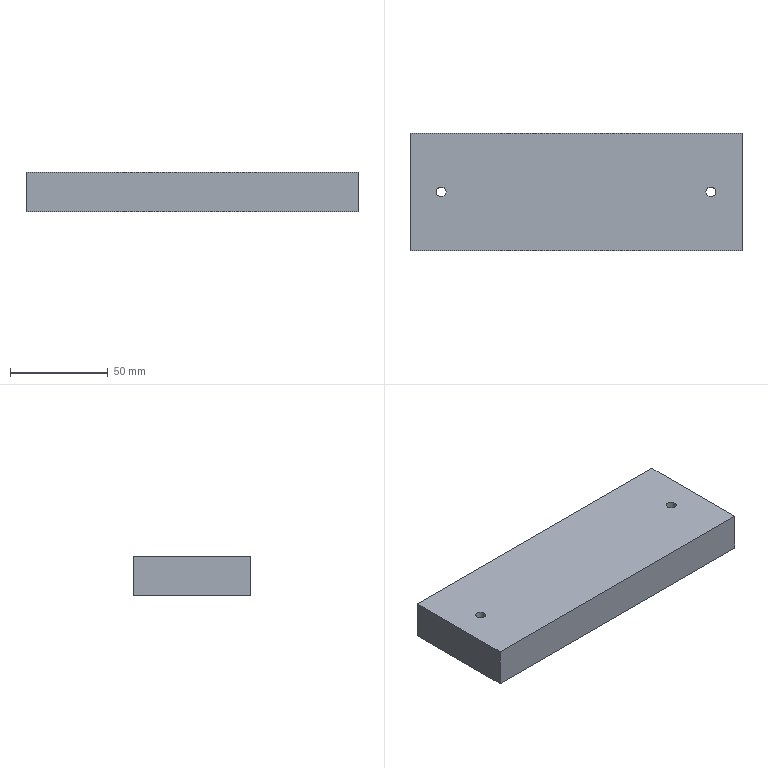Part | NX | 1 solid | 24 faces | box 170 x 60 x 20 mm | volume 202900 mm3 | plane 10 | torus 8 | cone 4 | cylinder 2 | commonest cylinder face diameters 5 x2
STEP:
#1=CARTESIAN_POINT('',(-85.,30.,1.5));
#2=VERTEX_POINT('',#1);
#3=CARTESIAN_POINT('',(-85.,-30.,1.5));
#4=VERTEX_POINT('',#3);
#5=CARTESIAN_POINT('',(-85.,28.565,1.5));
#6=DIRECTION('',(0.,-1.,0.));
#7=VECTOR('',#6,1000.);
#8=LINE('',#5,#7);
#9=EDGE_CURVE('',#2,#4,#8,.T.);
#10=ORIENTED_EDGE('',*,*,#9,.T.);
#11=CARTESIAN_POINT('',(-85.,-30.,21.5));
#12=VERTEX_POINT('',#11);
#13=CARTESIAN_POINT('',(-85.,-30.,1.5));
#14=DIRECTION('',(0.,0.,1.));
#15=VECTOR('',#14,1000.);
#16=LINE('',#13,#15);
#17=EDGE_CURVE('',#4,#12,#16,.T.);
#18=ORIENTED_EDGE('',*,*,#17,.T.);
#19=CARTESIAN_POINT('',(-85.,30.,21.5));
#20=VERTEX_POINT('',#19);
#21=CARTESIAN_POINT('',(-85.,0.,21.5));
#22=DIRECTION('',(0.,1.,0.));
#23=VECTOR('',#22,1000.);
#24=LINE('',#21,#23);
#25=EDGE_CURVE('',#12,#20,#24,.T.);
#26=ORIENTED_EDGE('',*,*,#25,.T.);
#27=CARTESIAN_POINT('',(-85.,30.,1.5));
#28=DIRECTION('',(0.,0.,1.));
#29=VECTOR('',#28,1000.);
#30=LINE('',#27,#29);
#31=EDGE_CURVE('',#2,#20,#30,.T.);
#32=ORIENTED_EDGE('',*,*,#31,.F.);
#33=EDGE_LOOP('',(#10,#18,#26,#32));
#34=FACE_BOUND('',#33,.T.);
#35=CARTESIAN_POINT('',(-85.,0.,1.5));
#36=DIRECTION('',(-1.,0.,0.));
#37=DIRECTION('',(0.,0.,1.));
#38=AXIS2_PLACEMENT_3D('',#35,#36,#37);
#39=PLANE('',#38);
#40=ADVANCED_FACE('',(#34),#39,.T.);
#41=CARTESIAN_POINT('',(85.,-30.,1.5));
#42=VERTEX_POINT('',#41);
#43=CARTESIAN_POINT('',(85.,30.,1.5));
#44=VERTEX_POINT('',#43);
#45=CARTESIAN_POINT('',(85.,28.565,1.5));
#46=DIRECTION('',(0.,1.,0.));
#47=VECTOR('',#46,1000.);
#48=LINE('',#45,#47);
#49=EDGE_CURVE('',#42,#44,#48,.T.);
#50=ORIENTED_EDGE('',*,*,#49,.T.);
#51=CARTESIAN_POINT('',(85.,30.,21.5));
#52=VERTEX_POINT('',#51);
#53=CARTESIAN_POINT('',(85.,30.,1.5));
#54=DIRECTION('',(0.,0.,1.));
#55=VECTOR('',#54,1000.);
#56=LINE('',#53,#55);
#57=EDGE_CURVE('',#44,#52,#56,.T.);
#58=ORIENTED_EDGE('',*,*,#57,.T.);
#59=CARTESIAN_POINT('',(85.,-30.,21.5));
#60=VERTEX_POINT('',#59);
#61=CARTESIAN_POINT('',(85.,0.,21.5));
#62=DIRECTION('',(0.,-1.,0.));
#63=VECTOR('',#62,1000.);
#64=LINE('',#61,#63);
#65=EDGE_CURVE('',#52,#60,#64,.T.);
#66=ORIENTED_EDGE('',*,*,#65,.T.);
#67=CARTESIAN_POINT('',(85.,-30.,1.5));
#68=DIRECTION('',(0.,0.,1.));
#69=VECTOR('',#68,1000.);
#70=LINE('',#67,#69);
#71=EDGE_CURVE('',#42,#60,#70,.T.);
#72=ORIENTED_EDGE('',*,*,#71,.F.);
#73=EDGE_LOOP('',(#50,#58,#66,#72));
#74=FACE_BOUND('',#73,.T.);
#75=CARTESIAN_POINT('',(85.,0.,1.5));
#76=DIRECTION('',(1.,0.,0.));
#77=DIRECTION('',(0.,0.,-1.));
#78=AXIS2_PLACEMENT_3D('',#75,#76,#77);
#79=PLANE('',#78);
#80=ADVANCED_FACE('',(#74),#79,.T.);
#81=CARTESIAN_POINT('',(71.5,0.,21.5));
#82=VERTEX_POINT('',#81);
#83=CARTESIAN_POINT('',(69.,0.,21.5));
#84=DIRECTION('',(0.,0.,1.));
#85=DIRECTION('',(1.,0.,0.));
#86=AXIS2_PLACEMENT_3D('',#83,#84,#85);
#87=CIRCLE('',#86,2.5);
#88=EDGE_CURVE('',#82,#82,#87,.F.);
#89=ORIENTED_EDGE('',*,*,#88,.T.);
#90=EDGE_LOOP('',(#89));
#91=FACE_BOUND('',#90,.T.);
#92=CARTESIAN_POINT('',(-66.5,0.,21.5));
#93=VERTEX_POINT('',#92);
#94=CARTESIAN_POINT('',(-69.,0.,21.5));
#95=DIRECTION('',(0.,0.,1.));
#96=DIRECTION('',(1.,0.,0.));
#97=AXIS2_PLACEMENT_3D('',#94,#95,#96);
#98=CIRCLE('',#97,2.5);
#99=EDGE_CURVE('',#93,#93,#98,.F.);
#100=ORIENTED_EDGE('',*,*,#99,.T.);
#101=EDGE_LOOP('',(#100));
#102=FACE_BOUND('',#101,.T.);
#103=CARTESIAN_POINT('',(0.,-30.,21.5));
#104=DIRECTION('',(-1.,0.,0.));
#105=VECTOR('',#104,1000.);
#106=LINE('',#103,#105);
#107=EDGE_CURVE('',#60,#12,#106,.T.);
#108=ORIENTED_EDGE('',*,*,#107,.F.);
#109=ORIENTED_EDGE('',*,*,#65,.F.);
#110=CARTESIAN_POINT('',(0.,30.,21.5));
#111=DIRECTION('',(1.,0.,0.));
#112=VECTOR('',#111,1000.);
#113=LINE('',#110,#112);
#114=EDGE_CURVE('',#20,#52,#113,.T.);
#115=ORIENTED_EDGE('',*,*,#114,.F.);
#116=ORIENTED_EDGE('',*,*,#25,.F.);
#117=EDGE_LOOP('',(#108,#109,#115,#116));
#118=FACE_BOUND('',#117,.T.);
#119=CARTESIAN_POINT('',(0.,0.,21.5));
#120=DIRECTION('',(0.,0.,1.));
#121=DIRECTION('',(1.,0.,0.));
#122=AXIS2_PLACEMENT_3D('',#119,#120,#121);
#123=PLANE('',#122);
#124=ADVANCED_FACE('',(#91,#102,#118),#123,.T.);
#125=CARTESIAN_POINT('',(-38.195,15.,1.5));
#126=VERTEX_POINT('',#125);
#127=CARTESIAN_POINT('',(-41.999,15.,1.5));
#128=DIRECTION('',(0.,0.,1.));
#129=DIRECTION('',(1.,0.,0.));
#130=AXIS2_PLACEMENT_3D('',#127,#128,#129);
#131=CIRCLE('',#130,3.804);
#132=EDGE_CURVE('',#126,#126,#131,.T.);
#133=ORIENTED_EDGE('',*,*,#132,.T.);
#134=EDGE_LOOP('',(#133));
#135=FACE_BOUND('',#134,.T.);
#136=CARTESIAN_POINT('',(45.805,15.,1.5));
#137=VERTEX_POINT('',#136);
#138=CARTESIAN_POINT('',(42.001,15.,1.5));
#139=DIRECTION('',(0.,0.,1.));
#140=DIRECTION('',(1.,0.,0.));
#141=AXIS2_PLACEMENT_3D('',#138,#139,#140);
#142=CIRCLE('',#141,3.804);
#143=EDGE_CURVE('',#137,#137,#142,.T.);
#144=ORIENTED_EDGE('',*,*,#143,.T.);
#145=EDGE_LOOP('',(#144));
#146=FACE_BOUND('',#145,.T.);
#147=CARTESIAN_POINT('',(28.805,-22.,1.5));
#148=VERTEX_POINT('',#147);
#149=CARTESIAN_POINT('',(25.001,-22.,1.5));
#150=DIRECTION('',(0.,0.,1.));
#151=DIRECTION('',(1.,0.,0.));
#152=AXIS2_PLACEMENT_3D('',#149,#150,#151);
#153=CIRCLE('',#152,3.804);
#154=EDGE_CURVE('',#148,#148,#153,.T.);
#155=ORIENTED_EDGE('',*,*,#154,.T.);
#156=EDGE_LOOP('',(#155));
#157=FACE_BOUND('',#156,.T.);
#158=CARTESIAN_POINT('',(-21.195,-22.,1.5));
#159=VERTEX_POINT('',#158);
#160=CARTESIAN_POINT('',(-24.999,-22.,1.5));
#161=DIRECTION('',(0.,0.,1.));
#162=DIRECTION('',(1.,0.,0.));
#163=AXIS2_PLACEMENT_3D('',#160,#161,#162);
#164=CIRCLE('',#163,3.804);
#165=EDGE_CURVE('',#159,#159,#164,.T.);
#166=ORIENTED_EDGE('',*,*,#165,.T.);
#167=EDGE_LOOP('',(#166));
#168=FACE_BOUND('',#167,.T.);
#169=CARTESIAN_POINT('',(71.5,0.,1.5));
#170=VERTEX_POINT('',#169);
#171=CARTESIAN_POINT('',(69.,0.,1.5));
#172=DIRECTION('',(0.,0.,1.));
#173=DIRECTION('',(1.,0.,0.));
#174=AXIS2_PLACEMENT_3D('',#171,#172,#173);
#175=CIRCLE('',#174,2.5);
#176=EDGE_CURVE('',#170,#170,#175,.T.);
#177=ORIENTED_EDGE('',*,*,#176,.T.);
#178=EDGE_LOOP('',(#177));
#179=FACE_BOUND('',#178,.T.);
#180=CARTESIAN_POINT('',(-66.5,0.,1.5));
#181=VERTEX_POINT('',#180);
#182=CARTESIAN_POINT('',(-69.,0.,1.5));
#183=DIRECTION('',(0.,0.,1.));
#184=DIRECTION('',(1.,0.,0.));
#185=AXIS2_PLACEMENT_3D('',#182,#183,#184);
#186=CIRCLE('',#185,2.5);
#187=EDGE_CURVE('',#181,#181,#186,.T.);
#188=ORIENTED_EDGE('',*,*,#187,.T.);
#189=EDGE_LOOP('',(#188));
#190=FACE_BOUND('',#189,.T.);
#191=CARTESIAN_POINT('',(0.,-30.,1.5));
#192=DIRECTION('',(1.,0.,0.));
#193=VECTOR('',#192,1000.);
#194=LINE('',#191,#193);
#195=EDGE_CURVE('',#4,#42,#194,.T.);
#196=ORIENTED_EDGE('',*,*,#195,.F.);
#197=ORIENTED_EDGE('',*,*,#9,.F.);
#198=CARTESIAN_POINT('',(0.,30.,1.5));
#199=DIRECTION('',(-1.,0.,0.));
#200=VECTOR('',#199,1000.);
#201=LINE('',#198,#200);
#202=EDGE_CURVE('',#44,#2,#201,.T.);
#203=ORIENTED_EDGE('',*,*,#202,.F.);
#204=ORIENTED_EDGE('',*,*,#49,.F.);
#205=EDGE_LOOP('',(#196,#197,#203,#204));
#206=FACE_BOUND('',#205,.T.);
#207=CARTESIAN_POINT('',(44.401,28.565,1.5));
#208=DIRECTION('',(0.,0.,1.));
#209=DIRECTION('',(1.,0.,0.));
#210=AXIS2_PLACEMENT_3D('',#207,#208,#209);
#211=PLANE('',#210);
#212=ADVANCED_FACE('',(#135,#146,#157,#168,#179,#190,#206),#211,.F.);
#213=CARTESIAN_POINT('',(-23.637,-22.,6.5));
#214=VERTEX_POINT('',#213);
#215=CARTESIAN_POINT('',(-24.999,-22.,6.5));
#216=DIRECTION('',(0.,0.,1.));
#217=DIRECTION('',(1.,0.,0.));
#218=AXIS2_PLACEMENT_3D('',#215,#216,#217);
#219=CIRCLE('',#218,1.363);
#220=EDGE_CURVE('',#214,#214,#219,.F.);
#221=ORIENTED_EDGE('',*,*,#220,.T.);
#222=EDGE_LOOP('',(#221));
#223=FACE_BOUND('',#222,.T.);
#224=CARTESIAN_POINT('',(-24.999,-22.,6.5));
#225=DIRECTION('',(0.,0.,1.));
#226=DIRECTION('',(0.,1.,0.));
#227=AXIS2_PLACEMENT_3D('',#224,#225,#226);
#228=PLANE('',#227);
#229=ADVANCED_FACE('',(#223),#228,.F.);
#230=CARTESIAN_POINT('',(-26.857,-22.,6.07));
#231=VERTEX_POINT('',#230);
#232=CARTESIAN_POINT('',(-24.999,-22.,6.07));
#233=DIRECTION('',(0.,0.,-1.));
#234=DIRECTION('',(-1.,0.,0.));
#235=AXIS2_PLACEMENT_3D('',#232,#233,#234);
#236=CIRCLE('',#235,1.858);
#237=EDGE_CURVE('',#231,#231,#236,.F.);
#238=ORIENTED_EDGE('',*,*,#237,.T.);
#239=EDGE_LOOP('',(#238));
#240=FACE_BOUND('',#239,.T.);
#241=CARTESIAN_POINT('',(-22.681,-22.,2.791));
#242=VERTEX_POINT('',#241);
#243=CARTESIAN_POINT('',(-24.999,-22.,2.791));
#244=DIRECTION('',(0.,0.,1.));
#245=DIRECTION('',(1.,0.,0.));
#246=AXIS2_PLACEMENT_3D('',#243,#244,#245);
#247=CIRCLE('',#246,2.319);
#248=EDGE_CURVE('',#242,#242,#247,.F.);
#249=ORIENTED_EDGE('',*,*,#248,.T.);
#250=EDGE_LOOP('',(#249));
#251=FACE_BOUND('',#250,.T.);
#252=CARTESIAN_POINT('',(-24.999,-22.,1.5));
#253=DIRECTION('',(0.,0.,-1.));
#254=DIRECTION('',(0.,1.,0.));
#255=AXIS2_PLACEMENT_3D('',#252,#253,#254);
#256=CONICAL_SURFACE('',#255,2.5,0.1396);
#257=ADVANCED_FACE('',(#240,#251),#256,.F.);
#258=CARTESIAN_POINT('',(26.363,-22.,6.5));
#259=VERTEX_POINT('',#258);
#260=CARTESIAN_POINT('',(25.001,-22.,6.5));
#261=DIRECTION('',(0.,0.,1.));
#262=DIRECTION('',(1.,0.,0.));
#263=AXIS2_PLACEMENT_3D('',#260,#261,#262);
#264=CIRCLE('',#263,1.363);
#265=EDGE_CURVE('',#259,#259,#264,.F.);
#266=ORIENTED_EDGE('',*,*,#265,.T.);
#267=EDGE_LOOP('',(#266));
#268=FACE_BOUND('',#267,.T.);
#269=CARTESIAN_POINT('',(25.001,-22.,6.5));
#270=DIRECTION('',(0.,0.,1.));
#271=DIRECTION('',(0.,1.,0.));
#272=AXIS2_PLACEMENT_3D('',#269,#270,#271);
#273=PLANE('',#272);
#274=ADVANCED_FACE('',(#268),#273,.F.);
#275=CARTESIAN_POINT('',(23.143,-22.,6.07));
#276=VERTEX_POINT('',#275);
#277=CARTESIAN_POINT('',(25.001,-22.,6.07));
#278=DIRECTION('',(0.,0.,-1.));
#279=DIRECTION('',(-1.,0.,0.));
#280=AXIS2_PLACEMENT_3D('',#277,#278,#279);
#281=CIRCLE('',#280,1.858);
#282=EDGE_CURVE('',#276,#276,#281,.F.);
#283=ORIENTED_EDGE('',*,*,#282,.T.);
#284=EDGE_LOOP('',(#283));
#285=FACE_BOUND('',#284,.T.);
#286=CARTESIAN_POINT('',(27.319,-22.,2.791));
#287=VERTEX_POINT('',#286);
#288=CARTESIAN_POINT('',(25.001,-22.,2.791));
#289=DIRECTION('',(0.,0.,1.));
#290=DIRECTION('',(1.,0.,0.));
#291=AXIS2_PLACEMENT_3D('',#288,#289,#290);
#292=CIRCLE('',#291,2.319);
#293=EDGE_CURVE('',#287,#287,#292,.F.);
#294=ORIENTED_EDGE('',*,*,#293,.T.);
#295=EDGE_LOOP('',(#294));
#296=FACE_BOUND('',#295,.T.);
#297=CARTESIAN_POINT('',(25.001,-22.,1.5));
#298=DIRECTION('',(0.,0.,-1.));
#299=DIRECTION('',(0.,1.,0.));
#300=AXIS2_PLACEMENT_3D('',#297,#298,#299);
#301=CONICAL_SURFACE('',#300,2.5,0.1396);
#302=ADVANCED_FACE('',(#285,#296),#301,.F.);
#303=CARTESIAN_POINT('',(40.638,15.,6.5));
#304=VERTEX_POINT('',#303);
#305=CARTESIAN_POINT('',(42.001,15.,6.5));
#306=DIRECTION('',(0.,0.,-1.));
#307=DIRECTION('',(-1.,0.,0.));
#308=AXIS2_PLACEMENT_3D('',#305,#306,#307);
#309=CIRCLE('',#308,1.363);
#310=EDGE_CURVE('',#304,#304,#309,.T.);
#311=ORIENTED_EDGE('',*,*,#310,.T.);
#312=EDGE_LOOP('',(#311));
#313=FACE_BOUND('',#312,.T.);
#314=CARTESIAN_POINT('',(42.001,15.,6.5));
#315=DIRECTION('',(0.,0.,-1.));
#316=DIRECTION('',(0.,-1.,0.));
#317=AXIS2_PLACEMENT_3D('',#314,#315,#316);
#318=PLANE('',#317);
#319=ADVANCED_FACE('',(#313),#318,.T.);
#320=CARTESIAN_POINT('',(43.859,15.,6.07));
#321=VERTEX_POINT('',#320);
#322=CARTESIAN_POINT('',(42.001,15.,6.07));
#323=DIRECTION('',(0.,0.,1.));
#324=DIRECTION('',(1.,0.,0.));
#325=AXIS2_PLACEMENT_3D('',#322,#323,#324);
#326=CIRCLE('',#325,1.858);
#327=EDGE_CURVE('',#321,#321,#326,.T.);
#328=ORIENTED_EDGE('',*,*,#327,.T.);
#329=EDGE_LOOP('',(#328));
#330=FACE_BOUND('',#329,.T.);
#331=CARTESIAN_POINT('',(44.319,15.,2.791));
#332=VERTEX_POINT('',#331);
#333=CARTESIAN_POINT('',(42.001,15.,2.791));
#334=DIRECTION('',(0.,0.,1.));
#335=DIRECTION('',(1.,0.,0.));
#336=AXIS2_PLACEMENT_3D('',#333,#334,#335);
#337=CIRCLE('',#336,2.319);
#338=EDGE_CURVE('',#332,#332,#337,.F.);
#339=ORIENTED_EDGE('',*,*,#338,.T.);
#340=EDGE_LOOP('',(#339));
#341=FACE_BOUND('',#340,.T.);
#342=CARTESIAN_POINT('',(42.001,15.,1.5));
#343=DIRECTION('',(0.,0.,-1.));
#344=DIRECTION('',(0.,1.,0.));
#345=AXIS2_PLACEMENT_3D('',#342,#343,#344);
#346=CONICAL_SURFACE('',#345,2.5,0.1396);
#347=ADVANCED_FACE('',(#330,#341),#346,.F.);
#348=CARTESIAN_POINT('',(-40.637,15.,6.5));
#349=VERTEX_POINT('',#348);
#350=CARTESIAN_POINT('',(-41.999,15.,6.5));
#351=DIRECTION('',(0.,0.,1.));
#352=DIRECTION('',(1.,0.,0.));
#353=AXIS2_PLACEMENT_3D('',#350,#351,#352);
#354=CIRCLE('',#353,1.363);
#355=EDGE_CURVE('',#349,#349,#354,.F.);
#356=ORIENTED_EDGE('',*,*,#355,.T.);
#357=EDGE_LOOP('',(#356));
#358=FACE_BOUND('',#357,.T.);
#359=CARTESIAN_POINT('',(-41.999,15.,6.5));
#360=DIRECTION('',(0.,0.,1.));
#361=DIRECTION('',(0.,1.,0.));
#362=AXIS2_PLACEMENT_3D('',#359,#360,#361);
#363=PLANE('',#362);
#364=ADVANCED_FACE('',(#358),#363,.F.);
#365=CARTESIAN_POINT('',(-43.857,15.,6.07));
#366=VERTEX_POINT('',#365);
#367=CARTESIAN_POINT('',(-41.999,15.,6.07));
#368=DIRECTION('',(0.,0.,-1.));
#369=DIRECTION('',(-1.,0.,0.));
#370=AXIS2_PLACEMENT_3D('',#367,#368,#369);
#371=CIRCLE('',#370,1.858);
#372=EDGE_CURVE('',#366,#366,#371,.F.);
#373=ORIENTED_EDGE('',*,*,#372,.T.);
#374=EDGE_LOOP('',(#373));
#375=FACE_BOUND('',#374,.T.);
#376=CARTESIAN_POINT('',(-39.681,15.,2.791));
#377=VERTEX_POINT('',#376);
#378=CARTESIAN_POINT('',(-41.999,15.,2.791));
#379=DIRECTION('',(0.,0.,1.));
#380=DIRECTION('',(1.,0.,0.));
#381=AXIS2_PLACEMENT_3D('',#378,#379,#380);
#382=CIRCLE('',#381,2.319);
#383=EDGE_CURVE('',#377,#377,#382,.F.);
#384=ORIENTED_EDGE('',*,*,#383,.T.);
#385=EDGE_LOOP('',(#384));
#386=FACE_BOUND('',#385,.T.);
#387=CARTESIAN_POINT('',(-41.999,15.,1.5));
#388=DIRECTION('',(0.,0.,-1.));
#389=DIRECTION('',(0.,1.,0.));
#390=AXIS2_PLACEMENT_3D('',#387,#388,#389);
#391=CONICAL_SURFACE('',#390,2.5,0.1396);
#392=ADVANCED_FACE('',(#375,#386),#391,.F.);
#393=ORIENTED_EDGE('',*,*,#31,.T.);
#394=ORIENTED_EDGE('',*,*,#114,.T.);
#395=ORIENTED_EDGE('',*,*,#57,.F.);
#396=ORIENTED_EDGE('',*,*,#202,.T.);
#397=EDGE_LOOP('',(#393,#394,#395,#396));
#398=FACE_BOUND('',#397,.T.);
#399=CARTESIAN_POINT('',(0.,30.,1.5));
#400=DIRECTION('',(0.,1.,0.));
#401=DIRECTION('',(0.,0.,1.));
#402=AXIS2_PLACEMENT_3D('',#399,#400,#401);
#403=PLANE('',#402);
#404=ADVANCED_FACE('',(#398),#403,.T.);
#405=ORIENTED_EDGE('',*,*,#71,.T.);
#406=ORIENTED_EDGE('',*,*,#107,.T.);
#407=ORIENTED_EDGE('',*,*,#17,.F.);
#408=ORIENTED_EDGE('',*,*,#195,.T.);
#409=EDGE_LOOP('',(#405,#406,#407,#408));
#410=FACE_BOUND('',#409,.T.);
#411=CARTESIAN_POINT('',(0.,-30.,1.5));
#412=DIRECTION('',(0.,-1.,0.));
#413=DIRECTION('',(0.,0.,-1.));
#414=AXIS2_PLACEMENT_3D('',#411,#412,#413);
#415=PLANE('',#414);
#416=ADVANCED_FACE('',(#410),#415,.T.);
#417=ORIENTED_EDGE('',*,*,#99,.F.);
#418=EDGE_LOOP('',(#417));
#419=FACE_BOUND('',#418,.T.);
#420=ORIENTED_EDGE('',*,*,#187,.F.);
#421=EDGE_LOOP('',(#420));
#422=FACE_BOUND('',#421,.T.);
#423=CARTESIAN_POINT('',(-69.,0.,41.5));
#424=DIRECTION('',(0.,0.,-1.));
#425=DIRECTION('',(-1.,0.,0.));
#426=AXIS2_PLACEMENT_3D('',#423,#424,#425);
#427=CYLINDRICAL_SURFACE('',#426,2.5);
#428=ADVANCED_FACE('',(#419,#422),#427,.F.);
#429=ORIENTED_EDGE('',*,*,#88,.F.);
#430=EDGE_LOOP('',(#429));
#431=FACE_BOUND('',#430,.T.);
#432=ORIENTED_EDGE('',*,*,#176,.F.);
#433=EDGE_LOOP('',(#432));
#434=FACE_BOUND('',#433,.T.);
#435=CARTESIAN_POINT('',(69.,0.,41.5));
#436=DIRECTION('',(0.,0.,-1.));
#437=DIRECTION('',(-1.,0.,0.));
#438=AXIS2_PLACEMENT_3D('',#435,#436,#437);
#439=CYLINDRICAL_SURFACE('',#438,2.5);
#440=ADVANCED_FACE('',(#431,#434),#439,.F.);
#441=ORIENTED_EDGE('',*,*,#132,.F.);
#442=EDGE_LOOP('',(#441));
#443=FACE_BOUND('',#442,.T.);
#444=ORIENTED_EDGE('',*,*,#383,.F.);
#445=EDGE_LOOP('',(#444));
#446=FACE_BOUND('',#445,.T.);
#447=CARTESIAN_POINT('',(-41.999,15.,3.));
#448=DIRECTION('',(0.,0.,1.));
#449=DIRECTION('',(1.,0.,0.));
#450=AXIS2_PLACEMENT_3D('',#447,#448,#449);
#451=TOROIDAL_SURFACE('',#450,3.804,1.5);
#452=ADVANCED_FACE('',(#443,#446),#451,.T.);
#453=ORIENTED_EDGE('',*,*,#143,.F.);
#454=EDGE_LOOP('',(#453));
#455=FACE_BOUND('',#454,.T.);
#456=ORIENTED_EDGE('',*,*,#338,.F.);
#457=EDGE_LOOP('',(#456));
#458=FACE_BOUND('',#457,.T.);
#459=CARTESIAN_POINT('',(42.001,15.,3.));
#460=DIRECTION('',(0.,0.,1.));
#461=DIRECTION('',(1.,0.,0.));
#462=AXIS2_PLACEMENT_3D('',#459,#460,#461);
#463=TOROIDAL_SURFACE('',#462,3.804,1.5);
#464=ADVANCED_FACE('',(#455,#458),#463,.T.);
#465=ORIENTED_EDGE('',*,*,#154,.F.);
#466=EDGE_LOOP('',(#465));
#467=FACE_BOUND('',#466,.T.);
#468=ORIENTED_EDGE('',*,*,#293,.F.);
#469=EDGE_LOOP('',(#468));
#470=FACE_BOUND('',#469,.T.);
#471=CARTESIAN_POINT('',(25.001,-22.,3.));
#472=DIRECTION('',(0.,0.,1.));
#473=DIRECTION('',(1.,0.,0.));
#474=AXIS2_PLACEMENT_3D('',#471,#472,#473);
#475=TOROIDAL_SURFACE('',#474,3.804,1.5);
#476=ADVANCED_FACE('',(#467,#470),#475,.T.);
#477=ORIENTED_EDGE('',*,*,#165,.F.);
#478=EDGE_LOOP('',(#477));
#479=FACE_BOUND('',#478,.T.);
#480=ORIENTED_EDGE('',*,*,#248,.F.);
#481=EDGE_LOOP('',(#480));
#482=FACE_BOUND('',#481,.T.);
#483=CARTESIAN_POINT('',(-24.999,-22.,3.));
#484=DIRECTION('',(0.,0.,1.));
#485=DIRECTION('',(1.,0.,0.));
#486=AXIS2_PLACEMENT_3D('',#483,#484,#485);
#487=TOROIDAL_SURFACE('',#486,3.804,1.5);
#488=ADVANCED_FACE('',(#479,#482),#487,.T.);
#489=ORIENTED_EDGE('',*,*,#282,.F.);
#490=EDGE_LOOP('',(#489));
#491=FACE_BOUND('',#490,.T.);
#492=ORIENTED_EDGE('',*,*,#265,.F.);
#493=EDGE_LOOP('',(#492));
#494=FACE_BOUND('',#493,.T.);
#495=CARTESIAN_POINT('',(25.001,-22.,6.));
#496=DIRECTION('',(0.,0.,1.));
#497=DIRECTION('',(1.,0.,0.));
#498=AXIS2_PLACEMENT_3D('',#495,#496,#497);
#499=TOROIDAL_SURFACE('',#498,1.363,0.5);
#500=ADVANCED_FACE('',(#491,#494),#499,.F.);
#501=ORIENTED_EDGE('',*,*,#237,.F.);
#502=EDGE_LOOP('',(#501));
#503=FACE_BOUND('',#502,.T.);
#504=ORIENTED_EDGE('',*,*,#220,.F.);
#505=EDGE_LOOP('',(#504));
#506=FACE_BOUND('',#505,.T.);
#507=CARTESIAN_POINT('',(-24.999,-22.,6.));
#508=DIRECTION('',(0.,0.,1.));
#509=DIRECTION('',(1.,0.,0.));
#510=AXIS2_PLACEMENT_3D('',#507,#508,#509);
#511=TOROIDAL_SURFACE('',#510,1.363,0.5);
#512=ADVANCED_FACE('',(#503,#506),#511,.F.);
#513=ORIENTED_EDGE('',*,*,#310,.F.);
#514=EDGE_LOOP('',(#513));
#515=FACE_BOUND('',#514,.T.);
#516=ORIENTED_EDGE('',*,*,#327,.F.);
#517=EDGE_LOOP('',(#516));
#518=FACE_BOUND('',#517,.T.);
#519=CARTESIAN_POINT('',(42.001,15.,6.));
#520=DIRECTION('',(0.,0.,-1.));
#521=DIRECTION('',(-1.,0.,0.));
#522=AXIS2_PLACEMENT_3D('',#519,#520,#521);
#523=TOROIDAL_SURFACE('',#522,1.363,0.5);
#524=ADVANCED_FACE('',(#515,#518),#523,.F.);
#525=ORIENTED_EDGE('',*,*,#372,.F.);
#526=EDGE_LOOP('',(#525));
#527=FACE_BOUND('',#526,.T.);
#528=ORIENTED_EDGE('',*,*,#355,.F.);
#529=EDGE_LOOP('',(#528));
#530=FACE_BOUND('',#529,.T.);
#531=CARTESIAN_POINT('',(-41.999,15.,6.));
#532=DIRECTION('',(0.,0.,1.));
#533=DIRECTION('',(1.,0.,0.));
#534=AXIS2_PLACEMENT_3D('',#531,#532,#533);
#535=TOROIDAL_SURFACE('',#534,1.363,0.5);
#536=ADVANCED_FACE('',(#527,#530),#535,.F.);
#537=CLOSED_SHELL('',(#40,#80,#124,#212,#229,#257,#274,#302,#319,#347,#364,#392,#404,#416,#428,#440,#452,#464,#476,#488,#500,#512,#524,#536));
#538=MANIFOLD_SOLID_BREP('',#537);
#539=(LENGTH_UNIT()NAMED_UNIT(*)SI_UNIT(.MILLI.,.METRE.));
#540=UNCERTAINTY_MEASURE_WITH_UNIT(LENGTH_MEASURE(0.00001),#539,'','');
#541=(NAMED_UNIT(*)PLANE_ANGLE_UNIT()SI_UNIT($,.RADIAN.));
#542=(NAMED_UNIT(*)SI_UNIT($,.STERADIAN.)SOLID_ANGLE_UNIT());
#543=(GEOMETRIC_REPRESENTATION_CONTEXT(3)GLOBAL_UNCERTAINTY_ASSIGNED_CONTEXT((#540))GLOBAL_UNIT_ASSIGNED_CONTEXT((#539,#541,#542))REPRESENTATION_CONTEXT('',''));
#544=ADVANCED_BREP_SHAPE_REPRESENTATION('',(#538),#543);